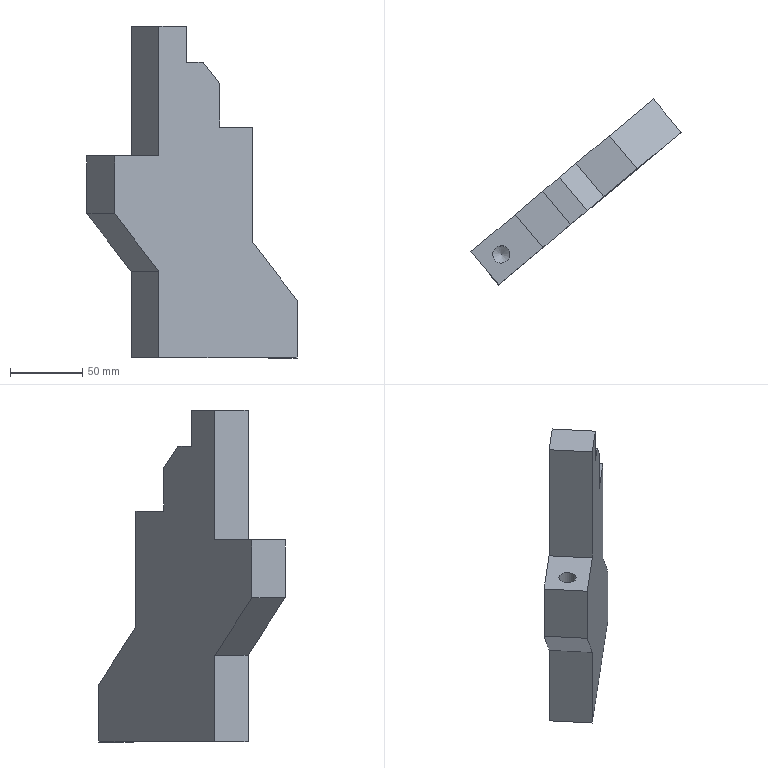Part | NX | features solid 2 | 1 solid | 19 faces | box 145.681 x 129.041 x 230 mm | volume 638662 mm3 | plane 17 | cone 1 | cylinder 1 | commonest cylinder face diameters 12 x1
STEP:
#1=CARTESIAN_POINT('',(765.783,315.367,-170.));
#2=VERTEX_POINT('',#1);
#3=CARTESIAN_POINT('',(765.783,315.367,-230.));
#4=VERTEX_POINT('',#3);
#5=CARTESIAN_POINT('',(765.783,315.367,0.));
#6=DIRECTION('',(0.,0.,-1.));
#7=VECTOR('',#6,1000.);
#8=LINE('',#5,#7);
#9=EDGE_CURVE('',#2,#4,#8,.T.);
#10=ORIENTED_EDGE('',*,*,#9,.F.);
#11=CARTESIAN_POINT('',(746.499,338.348,-170.));
#12=VERTEX_POINT('',#11);
#13=CARTESIAN_POINT('',(809.171,263.659,-170.));
#14=DIRECTION('',(-0.6428,0.766,0.));
#15=VECTOR('',#14,1000.);
#16=LINE('',#13,#15);
#17=EDGE_CURVE('',#2,#12,#16,.T.);
#18=ORIENTED_EDGE('',*,*,#17,.T.);
#19=CARTESIAN_POINT('',(746.499,338.348,-230.));
#20=VERTEX_POINT('',#19);
#21=CARTESIAN_POINT('',(746.499,338.348,0.));
#22=DIRECTION('',(0.,0.,-1.));
#23=VECTOR('',#22,1000.);
#24=LINE('',#21,#23);
#25=EDGE_CURVE('',#12,#20,#24,.T.);
#26=ORIENTED_EDGE('',*,*,#25,.T.);
#27=CARTESIAN_POINT('',(862.201,200.46,-230.));
#28=DIRECTION('',(-0.6428,0.766,0.));
#29=VECTOR('',#28,1000.);
#30=LINE('',#27,#29);
#31=EDGE_CURVE('',#4,#20,#30,.T.);
#32=ORIENTED_EDGE('',*,*,#31,.F.);
#33=EDGE_LOOP('',(#10,#18,#26,#32));
#34=FACE_BOUND('',#33,.T.);
#35=CARTESIAN_POINT('',(862.201,200.46,0.));
#36=DIRECTION('',(-0.766,-0.6428,0.));
#37=DIRECTION('',(0.,0.,-1.));
#38=AXIS2_PLACEMENT_3D('',#35,#36,#37);
#39=PLANE('',#38);
#40=ADVANCED_FACE('',(#34),#39,.T.);
#41=CARTESIAN_POINT('',(842.255,418.696,-190.));
#42=VERTEX_POINT('',#41);
#43=CARTESIAN_POINT('',(842.255,418.696,-230.));
#44=VERTEX_POINT('',#43);
#45=CARTESIAN_POINT('',(842.255,418.696,0.));
#46=DIRECTION('',(0.,0.,-1.));
#47=VECTOR('',#46,1000.);
#48=LINE('',#45,#47);
#49=EDGE_CURVE('',#42,#44,#48,.T.);
#50=ORIENTED_EDGE('',*,*,#49,.F.);
#51=CARTESIAN_POINT('',(861.539,395.715,-190.));
#52=VERTEX_POINT('',#51);
#53=CARTESIAN_POINT('',(861.539,395.715,-190.));
#54=DIRECTION('',(0.6428,-0.766,0.));
#55=VECTOR('',#54,1000.);
#56=LINE('',#53,#55);
#57=EDGE_CURVE('',#42,#52,#56,.T.);
#58=ORIENTED_EDGE('',*,*,#57,.T.);
#59=CARTESIAN_POINT('',(861.539,395.715,-230.));
#60=VERTEX_POINT('',#59);
#61=CARTESIAN_POINT('',(861.539,395.715,0.));
#62=DIRECTION('',(0.,0.,-1.));
#63=VECTOR('',#62,1000.);
#64=LINE('',#61,#63);
#65=EDGE_CURVE('',#52,#60,#64,.T.);
#66=ORIENTED_EDGE('',*,*,#65,.T.);
#67=CARTESIAN_POINT('',(867.967,388.055,-230.));
#68=DIRECTION('',(-0.6428,0.766,0.));
#69=VECTOR('',#68,1000.);
#70=LINE('',#67,#69);
#71=EDGE_CURVE('',#60,#44,#70,.T.);
#72=ORIENTED_EDGE('',*,*,#71,.T.);
#73=EDGE_LOOP('',(#50,#58,#66,#72));
#74=FACE_BOUND('',#73,.T.);
#75=CARTESIAN_POINT('',(867.967,388.055,0.));
#76=DIRECTION('',(-0.766,-0.6428,0.));
#77=DIRECTION('',(0.,0.,-1.));
#78=AXIS2_PLACEMENT_3D('',#75,#76,#77);
#79=PLANE('',#78);
#80=ADVANCED_FACE('',(#74),#79,.F.);
#81=CARTESIAN_POINT('',(811.613,392.985,-150.));
#82=VERTEX_POINT('',#81);
#83=CARTESIAN_POINT('',(811.613,392.985,-70.));
#84=VERTEX_POINT('',#83);
#85=CARTESIAN_POINT('',(811.613,392.985,-170.));
#86=DIRECTION('',(0.,0.,1.));
#87=VECTOR('',#86,1000.);
#88=LINE('',#85,#87);
#89=EDGE_CURVE('',#82,#84,#88,.T.);
#90=ORIENTED_EDGE('',*,*,#89,.F.);
#91=CARTESIAN_POINT('',(811.613,392.985,-150.));
#92=DIRECTION('',(0.5417,0.4545,-0.7071));
#93=VECTOR('',#92,1000.);
#94=LINE('',#91,#93);
#95=EDGE_CURVE('',#82,#42,#94,.T.);
#96=ORIENTED_EDGE('',*,*,#95,.T.);
#97=ORIENTED_EDGE('',*,*,#49,.T.);
#98=CARTESIAN_POINT('',(1190.805,711.165,-230.));
#99=DIRECTION('',(-0.766,-0.6428,0.));
#100=VECTOR('',#99,1000.);
#101=LINE('',#98,#100);
#102=EDGE_CURVE('',#44,#20,#101,.T.);
#103=ORIENTED_EDGE('',*,*,#102,.T.);
#104=ORIENTED_EDGE('',*,*,#25,.F.);
#105=CARTESIAN_POINT('',(715.858,312.636,-130.));
#106=VERTEX_POINT('',#105);
#107=CARTESIAN_POINT('',(953.331,511.901,-440.));
#108=DIRECTION('',(0.5417,0.4545,-0.7071));
#109=VECTOR('',#108,1000.);
#110=LINE('',#107,#109);
#111=EDGE_CURVE('',#12,#106,#110,.F.);
#112=ORIENTED_EDGE('',*,*,#111,.T.);
#113=CARTESIAN_POINT('',(715.858,312.636,-90.));
#114=VERTEX_POINT('',#113);
#115=CARTESIAN_POINT('',(715.858,312.636,-130.));
#116=DIRECTION('',(0.,0.,1.));
#117=VECTOR('',#116,1000.);
#118=LINE('',#115,#117);
#119=EDGE_CURVE('',#106,#114,#118,.T.);
#120=ORIENTED_EDGE('',*,*,#119,.T.);
#121=CARTESIAN_POINT('',(746.499,338.348,-90.));
#122=VERTEX_POINT('',#121);
#123=CARTESIAN_POINT('',(1190.805,711.165,-90.));
#124=DIRECTION('',(-0.766,-0.6428,0.));
#125=VECTOR('',#124,1000.);
#126=LINE('',#123,#125);
#127=EDGE_CURVE('',#122,#114,#126,.T.);
#128=ORIENTED_EDGE('',*,*,#127,.F.);
#129=CARTESIAN_POINT('',(746.499,338.348,0.));
#130=VERTEX_POINT('',#129);
#131=CARTESIAN_POINT('',(746.499,338.348,0.));
#132=DIRECTION('',(0.,0.,-1.));
#133=VECTOR('',#132,1000.);
#134=LINE('',#131,#133);
#135=EDGE_CURVE('',#130,#122,#134,.T.);
#136=ORIENTED_EDGE('',*,*,#135,.F.);
#137=CARTESIAN_POINT('',(765.651,354.418,0.));
#138=VERTEX_POINT('',#137);
#139=CARTESIAN_POINT('',(1190.805,711.165,0.));
#140=DIRECTION('',(-0.766,-0.6428,0.));
#141=VECTOR('',#140,1000.);
#142=LINE('',#139,#141);
#143=EDGE_CURVE('',#138,#130,#142,.T.);
#144=ORIENTED_EDGE('',*,*,#143,.F.);
#145=CARTESIAN_POINT('',(765.651,354.418,-25.));
#146=VERTEX_POINT('',#145);
#147=CARTESIAN_POINT('',(765.651,354.418,-30.));
#148=DIRECTION('',(0.,0.,1.));
#149=VECTOR('',#148,1000.);
#150=LINE('',#147,#149);
#151=EDGE_CURVE('',#146,#138,#150,.T.);
#152=ORIENTED_EDGE('',*,*,#151,.F.);
#153=CARTESIAN_POINT('',(777.141,364.059,-25.));
#154=VERTEX_POINT('',#153);
#155=CARTESIAN_POINT('',(842.255,418.696,-25.));
#156=DIRECTION('',(-0.766,-0.6428,0.));
#157=VECTOR('',#156,1000.);
#158=LINE('',#155,#157);
#159=EDGE_CURVE('',#154,#146,#158,.T.);
#160=ORIENTED_EDGE('',*,*,#159,.F.);
#161=CARTESIAN_POINT('',(788.632,373.701,-40.));
#162=VERTEX_POINT('',#161);
#163=CARTESIAN_POINT('',(777.141,364.059,-25.));
#164=DIRECTION('',(-0.5417,-0.4545,0.7071));
#165=VECTOR('',#164,1000.);
#166=LINE('',#163,#165);
#167=EDGE_CURVE('',#154,#162,#166,.F.);
#168=ORIENTED_EDGE('',*,*,#167,.T.);
#169=CARTESIAN_POINT('',(788.632,373.701,-70.));
#170=VERTEX_POINT('',#169);
#171=CARTESIAN_POINT('',(788.632,373.701,-70.));
#172=DIRECTION('',(0.,0.,1.));
#173=VECTOR('',#172,1000.);
#174=LINE('',#171,#173);
#175=EDGE_CURVE('',#170,#162,#174,.T.);
#176=ORIENTED_EDGE('',*,*,#175,.F.);
#177=CARTESIAN_POINT('',(842.255,418.696,-70.));
#178=DIRECTION('',(-0.766,-0.6428,0.));
#179=VECTOR('',#178,1000.);
#180=LINE('',#177,#179);
#181=EDGE_CURVE('',#84,#170,#180,.T.);
#182=ORIENTED_EDGE('',*,*,#181,.F.);
#183=EDGE_LOOP('',(#90,#96,#97,#103,#104,#112,#120,#128,#136,#144,#152,#160,#168,#176,#182));
#184=FACE_BOUND('',#183,.T.);
#185=CARTESIAN_POINT('',(1190.805,711.165,0.));
#186=DIRECTION('',(0.6428,-0.766,0.));
#187=DIRECTION('',(0.,0.,1.));
#188=AXIS2_PLACEMENT_3D('',#185,#186,#187);
#189=PLANE('',#188);
#190=ADVANCED_FACE('',(#184),#189,.F.);
#191=ORIENTED_EDGE('',*,*,#65,.F.);
#192=CARTESIAN_POINT('',(830.897,370.003,-150.));
#193=VERTEX_POINT('',#192);
#194=CARTESIAN_POINT('',(963.04,480.884,-322.5));
#195=DIRECTION('',(-0.5417,-0.4545,0.7071));
#196=VECTOR('',#195,1000.);
#197=LINE('',#194,#196);
#198=EDGE_CURVE('',#52,#193,#197,.T.);
#199=ORIENTED_EDGE('',*,*,#198,.T.);
#200=CARTESIAN_POINT('',(830.897,370.003,-70.));
#201=VERTEX_POINT('',#200);
#202=CARTESIAN_POINT('',(830.897,370.003,-170.));
#203=DIRECTION('',(0.,0.,1.));
#204=VECTOR('',#203,1000.);
#205=LINE('',#202,#204);
#206=EDGE_CURVE('',#193,#201,#205,.T.);
#207=ORIENTED_EDGE('',*,*,#206,.T.);
#208=CARTESIAN_POINT('',(807.916,350.72,-70.));
#209=VERTEX_POINT('',#208);
#210=CARTESIAN_POINT('',(861.539,395.715,-70.));
#211=DIRECTION('',(-0.766,-0.6428,0.));
#212=VECTOR('',#211,1000.);
#213=LINE('',#210,#212);
#214=EDGE_CURVE('',#201,#209,#213,.T.);
#215=ORIENTED_EDGE('',*,*,#214,.T.);
#216=CARTESIAN_POINT('',(807.916,350.72,-40.));
#217=VERTEX_POINT('',#216);
#218=CARTESIAN_POINT('',(807.916,350.72,-70.));
#219=DIRECTION('',(0.,0.,1.));
#220=VECTOR('',#219,1000.);
#221=LINE('',#218,#220);
#222=EDGE_CURVE('',#209,#217,#221,.T.);
#223=ORIENTED_EDGE('',*,*,#222,.T.);
#224=CARTESIAN_POINT('',(796.425,341.078,-25.));
#225=VERTEX_POINT('',#224);
#226=CARTESIAN_POINT('',(993.681,506.596,-282.5));
#227=DIRECTION('',(0.5417,0.4545,-0.7071));
#228=VECTOR('',#227,1000.);
#229=LINE('',#226,#228);
#230=EDGE_CURVE('',#217,#225,#229,.F.);
#231=ORIENTED_EDGE('',*,*,#230,.T.);
#232=CARTESIAN_POINT('',(784.934,331.436,-25.));
#233=VERTEX_POINT('',#232);
#234=CARTESIAN_POINT('',(861.539,395.715,-25.));
#235=DIRECTION('',(-0.766,-0.6428,0.));
#236=VECTOR('',#235,1000.);
#237=LINE('',#234,#236);
#238=EDGE_CURVE('',#225,#233,#237,.T.);
#239=ORIENTED_EDGE('',*,*,#238,.T.);
#240=CARTESIAN_POINT('',(784.934,331.436,0.));
#241=VERTEX_POINT('',#240);
#242=CARTESIAN_POINT('',(784.934,331.436,-30.));
#243=DIRECTION('',(0.,0.,1.));
#244=VECTOR('',#243,1000.);
#245=LINE('',#242,#244);
#246=EDGE_CURVE('',#233,#241,#245,.T.);
#247=ORIENTED_EDGE('',*,*,#246,.T.);
#248=CARTESIAN_POINT('',(765.783,315.367,0.));
#249=VERTEX_POINT('',#248);
#250=CARTESIAN_POINT('',(1210.089,688.183,0.));
#251=DIRECTION('',(-0.766,-0.6428,0.));
#252=VECTOR('',#251,1000.);
#253=LINE('',#250,#252);
#254=EDGE_CURVE('',#241,#249,#253,.T.);
#255=ORIENTED_EDGE('',*,*,#254,.T.);
#256=CARTESIAN_POINT('',(765.783,315.367,-90.));
#257=VERTEX_POINT('',#256);
#258=CARTESIAN_POINT('',(765.783,315.367,0.));
#259=DIRECTION('',(0.,0.,-1.));
#260=VECTOR('',#259,1000.);
#261=LINE('',#258,#260);
#262=EDGE_CURVE('',#249,#257,#261,.T.);
#263=ORIENTED_EDGE('',*,*,#262,.T.);
#264=CARTESIAN_POINT('',(735.141,289.655,-90.));
#265=VERTEX_POINT('',#264);
#266=CARTESIAN_POINT('',(1210.089,688.183,-90.));
#267=DIRECTION('',(-0.766,-0.6428,0.));
#268=VECTOR('',#267,1000.);
#269=LINE('',#266,#268);
#270=EDGE_CURVE('',#257,#265,#269,.T.);
#271=ORIENTED_EDGE('',*,*,#270,.T.);
#272=CARTESIAN_POINT('',(735.141,289.655,-130.));
#273=VERTEX_POINT('',#272);
#274=CARTESIAN_POINT('',(735.141,289.655,-130.));
#275=DIRECTION('',(0.,0.,1.));
#276=VECTOR('',#275,1000.);
#277=LINE('',#274,#276);
#278=EDGE_CURVE('',#273,#265,#277,.T.);
#279=ORIENTED_EDGE('',*,*,#278,.F.);
#280=CARTESIAN_POINT('',(765.783,315.367,-170.));
#281=DIRECTION('',(-0.5417,-0.4545,0.7071));
#282=VECTOR('',#281,1000.);
#283=LINE('',#280,#282);
#284=EDGE_CURVE('',#273,#2,#283,.F.);
#285=ORIENTED_EDGE('',*,*,#284,.T.);
#286=ORIENTED_EDGE('',*,*,#9,.T.);
#287=CARTESIAN_POINT('',(1210.089,688.183,-230.));
#288=DIRECTION('',(-0.766,-0.6428,0.));
#289=VECTOR('',#288,1000.);
#290=LINE('',#287,#289);
#291=EDGE_CURVE('',#60,#4,#290,.T.);
#292=ORIENTED_EDGE('',*,*,#291,.F.);
#293=EDGE_LOOP('',(#191,#199,#207,#215,#223,#231,#239,#247,#255,#263,#271,#279,#285,#286,#292));
#294=FACE_BOUND('',#293,.T.);
#295=CARTESIAN_POINT('',(1210.089,688.183,0.));
#296=DIRECTION('',(0.6428,-0.766,0.));
#297=DIRECTION('',(0.,0.,1.));
#298=AXIS2_PLACEMENT_3D('',#295,#296,#297);
#299=PLANE('',#298);
#300=ADVANCED_FACE('',(#294),#299,.T.);
#301=ORIENTED_EDGE('',*,*,#214,.F.);
#302=CARTESIAN_POINT('',(830.897,370.003,-70.));
#303=DIRECTION('',(-0.6428,0.766,0.));
#304=VECTOR('',#303,1000.);
#305=LINE('',#302,#304);
#306=EDGE_CURVE('',#201,#84,#305,.T.);
#307=ORIENTED_EDGE('',*,*,#306,.T.);
#308=ORIENTED_EDGE('',*,*,#181,.T.);
#309=CARTESIAN_POINT('',(807.916,350.72,-70.));
#310=DIRECTION('',(-0.6428,0.766,0.));
#311=VECTOR('',#310,1000.);
#312=LINE('',#309,#311);
#313=EDGE_CURVE('',#209,#170,#312,.T.);
#314=ORIENTED_EDGE('',*,*,#313,.F.);
#315=EDGE_LOOP('',(#301,#307,#308,#314));
#316=FACE_BOUND('',#315,.T.);
#317=CARTESIAN_POINT('',(842.255,418.696,-70.));
#318=DIRECTION('',(0.,0.,1.));
#319=DIRECTION('',(-0.766,-0.6428,0.));
#320=AXIS2_PLACEMENT_3D('',#317,#318,#319);
#321=PLANE('',#320);
#322=ADVANCED_FACE('',(#316),#321,.T.);
#323=ORIENTED_EDGE('',*,*,#238,.F.);
#324=CARTESIAN_POINT('',(796.425,341.078,-25.));
#325=DIRECTION('',(-0.6428,0.766,0.));
#326=VECTOR('',#325,1000.);
#327=LINE('',#324,#326);
#328=EDGE_CURVE('',#225,#154,#327,.T.);
#329=ORIENTED_EDGE('',*,*,#328,.T.);
#330=ORIENTED_EDGE('',*,*,#159,.T.);
#331=CARTESIAN_POINT('',(784.934,331.436,-25.));
#332=DIRECTION('',(-0.6428,0.766,0.));
#333=VECTOR('',#332,1000.);
#334=LINE('',#331,#333);
#335=EDGE_CURVE('',#233,#146,#334,.T.);
#336=ORIENTED_EDGE('',*,*,#335,.F.);
#337=EDGE_LOOP('',(#323,#329,#330,#336));
#338=FACE_BOUND('',#337,.T.);
#339=CARTESIAN_POINT('',(861.539,395.715,-25.));
#340=DIRECTION('',(0.,0.,1.));
#341=DIRECTION('',(-0.766,-0.6428,0.));
#342=AXIS2_PLACEMENT_3D('',#339,#340,#341);
#343=PLANE('',#342);
#344=ADVANCED_FACE('',(#338),#343,.T.);
#345=ORIENTED_EDGE('',*,*,#254,.F.);
#346=CARTESIAN_POINT('',(784.934,331.436,0.));
#347=DIRECTION('',(-0.6428,0.766,0.));
#348=VECTOR('',#347,1000.);
#349=LINE('',#346,#348);
#350=EDGE_CURVE('',#241,#138,#349,.T.);
#351=ORIENTED_EDGE('',*,*,#350,.T.);
#352=ORIENTED_EDGE('',*,*,#143,.T.);
#353=CARTESIAN_POINT('',(862.201,200.46,0.));
#354=DIRECTION('',(-0.6428,0.766,0.));
#355=VECTOR('',#354,1000.);
#356=LINE('',#353,#355);
#357=EDGE_CURVE('',#249,#130,#356,.T.);
#358=ORIENTED_EDGE('',*,*,#357,.F.);
#359=EDGE_LOOP('',(#345,#351,#352,#358));
#360=FACE_BOUND('',#359,.T.);
#361=CARTESIAN_POINT('',(1032.765,496.966,0.));
#362=DIRECTION('',(0.,0.,1.));
#363=DIRECTION('',(-0.766,-0.6428,0.));
#364=AXIS2_PLACEMENT_3D('',#361,#362,#363);
#365=PLANE('',#364);
#366=ADVANCED_FACE('',(#360),#365,.T.);
#367=CARTESIAN_POINT('',(862.201,200.46,-90.));
#368=DIRECTION('',(-0.6428,0.766,0.));
#369=VECTOR('',#368,1000.);
#370=LINE('',#367,#369);
#371=EDGE_CURVE('',#257,#122,#370,.T.);
#372=ORIENTED_EDGE('',*,*,#371,.F.);
#373=ORIENTED_EDGE('',*,*,#262,.F.);
#374=ORIENTED_EDGE('',*,*,#357,.T.);
#375=ORIENTED_EDGE('',*,*,#135,.T.);
#376=EDGE_LOOP('',(#372,#373,#374,#375));
#377=FACE_BOUND('',#376,.T.);
#378=CARTESIAN_POINT('',(862.201,200.46,0.));
#379=DIRECTION('',(-0.766,-0.6428,0.));
#380=DIRECTION('',(0.,0.,-1.));
#381=AXIS2_PLACEMENT_3D('',#378,#379,#380);
#382=PLANE('',#381);
#383=ADVANCED_FACE('',(#377),#382,.T.);
#384=ORIENTED_EDGE('',*,*,#71,.F.);
#385=ORIENTED_EDGE('',*,*,#291,.T.);
#386=ORIENTED_EDGE('',*,*,#31,.T.);
#387=ORIENTED_EDGE('',*,*,#102,.F.);
#388=EDGE_LOOP('',(#384,#385,#386,#387));
#389=FACE_BOUND('',#388,.T.);
#390=CARTESIAN_POINT('',(1032.765,496.966,-230.));
#391=DIRECTION('',(0.,0.,1.));
#392=DIRECTION('',(-0.766,-0.6428,0.));
#393=AXIS2_PLACEMENT_3D('',#390,#391,#392);
#394=PLANE('',#393);
#395=ADVANCED_FACE('',(#389),#394,.F.);
#396=ORIENTED_EDGE('',*,*,#350,.F.);
#397=ORIENTED_EDGE('',*,*,#246,.F.);
#398=ORIENTED_EDGE('',*,*,#335,.T.);
#399=ORIENTED_EDGE('',*,*,#151,.T.);
#400=EDGE_LOOP('',(#396,#397,#398,#399));
#401=FACE_BOUND('',#400,.T.);
#402=CARTESIAN_POINT('',(784.934,331.436,-30.));
#403=DIRECTION('',(0.766,0.6428,0.));
#404=DIRECTION('',(-0.6428,0.766,0.));
#405=AXIS2_PLACEMENT_3D('',#402,#403,#404);
#406=PLANE('',#405);
#407=ADVANCED_FACE('',(#401),#406,.T.);
#408=ORIENTED_EDGE('',*,*,#175,.T.);
#409=CARTESIAN_POINT('',(807.916,350.72,-40.));
#410=DIRECTION('',(0.6428,-0.766,0.));
#411=VECTOR('',#410,1000.);
#412=LINE('',#409,#411);
#413=EDGE_CURVE('',#162,#217,#412,.T.);
#414=ORIENTED_EDGE('',*,*,#413,.T.);
#415=ORIENTED_EDGE('',*,*,#222,.F.);
#416=ORIENTED_EDGE('',*,*,#313,.T.);
#417=EDGE_LOOP('',(#408,#414,#415,#416));
#418=FACE_BOUND('',#417,.T.);
#419=CARTESIAN_POINT('',(807.916,350.72,-70.));
#420=DIRECTION('',(0.766,0.6428,0.));
#421=DIRECTION('',(-0.6428,0.766,0.));
#422=AXIS2_PLACEMENT_3D('',#419,#420,#421);
#423=PLANE('',#422);
#424=ADVANCED_FACE('',(#418),#423,.T.);
#425=ORIENTED_EDGE('',*,*,#230,.F.);
#426=ORIENTED_EDGE('',*,*,#413,.F.);
#427=ORIENTED_EDGE('',*,*,#167,.F.);
#428=ORIENTED_EDGE('',*,*,#328,.F.);
#429=EDGE_LOOP('',(#425,#426,#427,#428));
#430=FACE_BOUND('',#429,.T.);
#431=CARTESIAN_POINT('',(796.425,341.078,-25.));
#432=DIRECTION('',(-0.5417,-0.4545,-0.7071));
#433=DIRECTION('',(0.5417,0.4545,-0.7071));
#434=AXIS2_PLACEMENT_3D('',#431,#432,#433);
#435=PLANE('',#434);
#436=ADVANCED_FACE('',(#430),#435,.F.);
#437=ORIENTED_EDGE('',*,*,#306,.F.);
#438=ORIENTED_EDGE('',*,*,#206,.F.);
#439=CARTESIAN_POINT('',(830.897,370.003,-150.));
#440=DIRECTION('',(-0.6428,0.766,0.));
#441=VECTOR('',#440,1000.);
#442=LINE('',#439,#441);
#443=EDGE_CURVE('',#193,#82,#442,.T.);
#444=ORIENTED_EDGE('',*,*,#443,.T.);
#445=ORIENTED_EDGE('',*,*,#89,.T.);
#446=EDGE_LOOP('',(#437,#438,#444,#445));
#447=FACE_BOUND('',#446,.T.);
#448=CARTESIAN_POINT('',(830.897,370.003,-170.));
#449=DIRECTION('',(0.766,0.6428,0.));
#450=DIRECTION('',(-0.6428,0.766,0.));
#451=AXIS2_PLACEMENT_3D('',#448,#449,#450);
#452=PLANE('',#451);
#453=ADVANCED_FACE('',(#447),#452,.T.);
#454=ORIENTED_EDGE('',*,*,#198,.F.);
#455=ORIENTED_EDGE('',*,*,#57,.F.);
#456=ORIENTED_EDGE('',*,*,#95,.F.);
#457=ORIENTED_EDGE('',*,*,#443,.F.);
#458=EDGE_LOOP('',(#454,#455,#456,#457));
#459=FACE_BOUND('',#458,.T.);
#460=CARTESIAN_POINT('',(830.897,370.003,-150.));
#461=DIRECTION('',(0.5417,0.4545,0.7071));
#462=DIRECTION('',(-0.5417,-0.4545,0.7071));
#463=AXIS2_PLACEMENT_3D('',#460,#461,#462);
#464=PLANE('',#463);
#465=ADVANCED_FACE('',(#459),#464,.T.);
#466=ORIENTED_EDGE('',*,*,#119,.F.);
#467=CARTESIAN_POINT('',(831.559,174.748,-130.));
#468=DIRECTION('',(0.6428,-0.766,0.));
#469=VECTOR('',#468,1000.);
#470=LINE('',#467,#469);
#471=EDGE_CURVE('',#106,#273,#470,.T.);
#472=ORIENTED_EDGE('',*,*,#471,.T.);
#473=ORIENTED_EDGE('',*,*,#278,.T.);
#474=CARTESIAN_POINT('',(831.559,174.748,-90.));
#475=DIRECTION('',(-0.6428,0.766,0.));
#476=VECTOR('',#475,1000.);
#477=LINE('',#474,#476);
#478=EDGE_CURVE('',#265,#114,#477,.T.);
#479=ORIENTED_EDGE('',*,*,#478,.T.);
#480=EDGE_LOOP('',(#466,#472,#473,#479));
#481=FACE_BOUND('',#480,.T.);
#482=CARTESIAN_POINT('',(831.559,174.748,-130.));
#483=DIRECTION('',(0.766,0.6428,0.));
#484=DIRECTION('',(0.,0.,1.));
#485=AXIS2_PLACEMENT_3D('',#482,#483,#484);
#486=PLANE('',#485);
#487=ADVANCED_FACE('',(#481),#486,.F.);
#488=CARTESIAN_POINT('',(742.967,310.265,-90.));
#489=VERTEX_POINT('',#488);
#490=CARTESIAN_POINT('',(736.99,310.788,-90.));
#491=DIRECTION('',(0.,0.,-1.));
#492=DIRECTION('',(0.9962,-0.08716,0.));
#493=AXIS2_PLACEMENT_3D('',#490,#491,#492);
#494=CIRCLE('',#493,6.);
#495=EDGE_CURVE('',#489,#489,#494,.T.);
#496=ORIENTED_EDGE('',*,*,#495,.T.);
#497=EDGE_LOOP('',(#496));
#498=FACE_BOUND('',#497,.T.);
#499=ORIENTED_EDGE('',*,*,#371,.T.);
#500=ORIENTED_EDGE('',*,*,#127,.T.);
#501=ORIENTED_EDGE('',*,*,#478,.F.);
#502=ORIENTED_EDGE('',*,*,#270,.F.);
#503=EDGE_LOOP('',(#499,#500,#501,#502));
#504=FACE_BOUND('',#503,.T.);
#505=CARTESIAN_POINT('',(1023.664,443.639,-90.));
#506=DIRECTION('',(0.,0.,1.));
#507=DIRECTION('',(-0.766,-0.6428,0.));
#508=AXIS2_PLACEMENT_3D('',#505,#506,#507);
#509=PLANE('',#508);
#510=ADVANCED_FACE('',(#498,#504),#509,.T.);
#511=ORIENTED_EDGE('',*,*,#284,.F.);
#512=ORIENTED_EDGE('',*,*,#471,.F.);
#513=ORIENTED_EDGE('',*,*,#111,.F.);
#514=ORIENTED_EDGE('',*,*,#17,.F.);
#515=EDGE_LOOP('',(#511,#512,#513,#514));
#516=FACE_BOUND('',#515,.T.);
#517=CARTESIAN_POINT('',(809.171,263.659,-170.));
#518=DIRECTION('',(0.5417,0.4545,0.7071));
#519=DIRECTION('',(-0.5417,-0.4545,0.7071));
#520=AXIS2_PLACEMENT_3D('',#517,#518,#519);
#521=PLANE('',#520);
#522=ADVANCED_FACE('',(#516),#521,.F.);
#523=CARTESIAN_POINT('',(742.967,310.265,-115.));
#524=VERTEX_POINT('',#523);
#525=CARTESIAN_POINT('',(736.99,310.788,-115.));
#526=DIRECTION('',(0.,0.,-1.));
#527=DIRECTION('',(0.9962,-0.08716,0.));
#528=AXIS2_PLACEMENT_3D('',#525,#526,#527);
#529=CIRCLE('',#528,6.);
#530=EDGE_CURVE('',#524,#524,#529,.T.);
#531=ORIENTED_EDGE('',*,*,#530,.F.);
#532=EDGE_LOOP('',(#531));
#533=FACE_BOUND('',#532,.T.);
#534=CARTESIAN_POINT('',(736.99,310.788,-118.605));
#535=VERTEX_POINT('',#534);
#536=VERTEX_LOOP('',#535);
#537=FACE_BOUND('',#536,.T.);
#538=CARTESIAN_POINT('',(736.99,310.788,-115.));
#539=DIRECTION('',(0.,0.,1.));
#540=DIRECTION('',(-0.9962,0.08716,0.));
#541=AXIS2_PLACEMENT_3D('',#538,#539,#540);
#542=CONICAL_SURFACE('',#541,6.,1.03);
#543=ADVANCED_FACE('',(#533,#537),#542,.F.);
#544=ORIENTED_EDGE('',*,*,#530,.T.);
#545=EDGE_LOOP('',(#544));
#546=FACE_BOUND('',#545,.T.);
#547=ORIENTED_EDGE('',*,*,#495,.F.);
#548=EDGE_LOOP('',(#547));
#549=FACE_BOUND('',#548,.T.);
#550=CARTESIAN_POINT('',(736.99,310.788,-90.));
#551=DIRECTION('',(0.,0.,-1.));
#552=DIRECTION('',(0.9962,-0.08716,0.));
#553=AXIS2_PLACEMENT_3D('',#550,#551,#552);
#554=CYLINDRICAL_SURFACE('',#553,6.);
#555=ADVANCED_FACE('',(#546,#549),#554,.F.);
#556=CLOSED_SHELL('',(#40,#80,#190,#300,#322,#344,#366,#383,#395,#407,#424,#436,#453,#465,#487,#510,#522,#543,#555));
#557=MANIFOLD_SOLID_BREP('',#556);
#558=(LENGTH_UNIT()NAMED_UNIT(*)SI_UNIT(.MILLI.,.METRE.));
#559=UNCERTAINTY_MEASURE_WITH_UNIT(LENGTH_MEASURE(0.00001),#558,'','');
#560=(NAMED_UNIT(*)PLANE_ANGLE_UNIT()SI_UNIT($,.RADIAN.));
#561=(NAMED_UNIT(*)SI_UNIT($,.STERADIAN.)SOLID_ANGLE_UNIT());
#562=(GEOMETRIC_REPRESENTATION_CONTEXT(3)GLOBAL_UNCERTAINTY_ASSIGNED_CONTEXT((#559))GLOBAL_UNIT_ASSIGNED_CONTEXT((#558,#560,#561))REPRESENTATION_CONTEXT('',''));
#563=ADVANCED_BREP_SHAPE_REPRESENTATION('',(#557),#562);